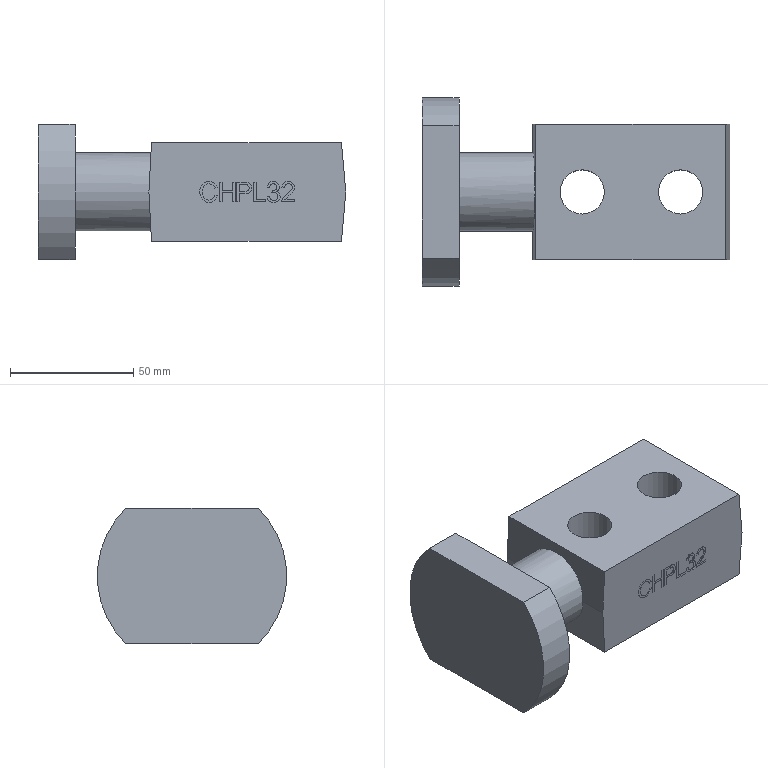Part | NX | features CHPL32_1 2 | 1 solid | 86 faces | box 125 x 77 x 55 mm | volume 234575 mm3 | plane 61 | cylinder 25 | commonest cylinder face diameters 4.823 x2 18 x2 77 x2 2.833 x1 2.919 x1 3.134 x1